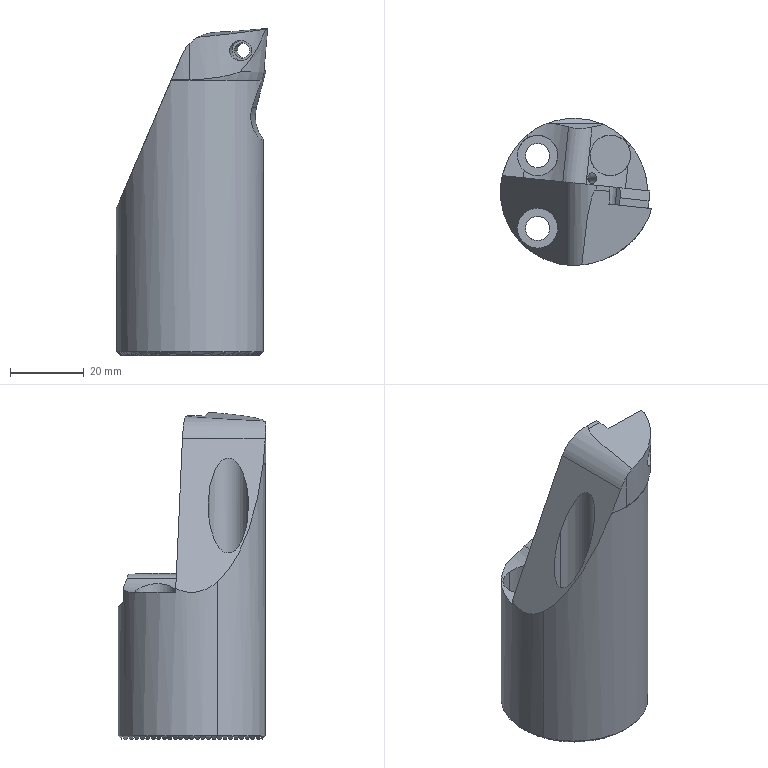NC program | Mastercam | posted with a generic post
Whole program:
%
:0001()
(MATERIAL - ALUMINUM MM - 2024)
(T10|50 FM/CTM |H10)
(T2|12 FEMR |H2|D2|WEAR COMP|TOOL DIA. - 12.|XY STOCK TO LEAVE - .3|Z STOCK TO LEAVE - 0.)
(T3|10 CHM |H3)
(T4|11 DR |H4)
(T11|6.6 DR |H11)
(T7|6 CBCHM |H7|D7|WEAR COMP|TOOL DIA. - 6.)
(T5|8 FEMR |H5|D5|WEAR COMP|TOOL DIA. - 8.|XY STOCK TO LEAVE - .05|Z STOCK TO LEAVE - .05)
(T6|8 FEMF |H6|D6|WEAR COMP|TOOL DIA. - 8.|XY STOCK TO LEAVE - .01|Z STOCK TO LEAVE - 0.)
(T8|26 60DTH |H8|D8|WEAR COMP|TOOL DIA. - 26.|XY STOCK TO LEAVE - .1|Z STOCK TO LEAVE - 0.)
(T13|11 DR |H13)
(T12|10.8 FL |H12)
N100 G21
N102 G0 G17 G40 G80 G90 G94 G98
N104 G0 G28 G91 Z0.
N106 G0 G28 X0. Y0.
(50 FM/CTM |TOOL - 10|DIA. OFF. - 10|LEN. - 10|TOOL DIA. - 50.)
N108 T10 M6
N110 G0 G54 G90 X0. Y-55. C0. B0. S1600 M3
N112 G43 H10 Z53.5
N114 Z4.5
N116 G1 Z0. F600.
N118 Y-20.
N120 Y20.
N122 Y55.
N124 G0 Z53.5
N126 M5
N128 G0 G28 G91 Z0.
N130 G28
N132 M01
N134 G0 G17 G40 G80 G90 G94 G98
N136 G0 G28 G91 Z0.
(12 FEMR |TOOL - 2|DIA. OFF. - 2|LEN. - 2|TOOL DIA. - 12.)
N138 T2 M6
N140 G0 G54 G90 X-1. Y35.7 C0. B0. S3500 M3
N142 G43 H2 Z50.
N144 Z1.
N146 G1 Z-1.5 F2000.
N148 G41 D2 Y27.3 F400.
N150 G3 X0. Y26.3 I1.
N152 G2 X26.3 Y0. J-26.3
N154 X0. Y-26.3 I-26.3
N156 X-26.3 Y0. J26.3
N158 X0. Y26.3 I26.3
N160 X.5 Y26.295 J-26.3
N162 G1 X.519
N164 G3 X1.519 Y27.276 J1.
N166 G1 G40 X1.678 Y35.675
N168 G0 Z50.
N170 M5
N172 G0 G28 G91 Z0.
N174 G28
N176 M01
N178 G0 G17 G40 G80 G90 G94 G98
N180 G0 G28 G91 Z0.
(10 CHM |TOOL - 3|DIA. OFF. - 3|LEN. - 3|TOOL DIA. - 10.)
N182 T3 M6
N184 G0 G54 G90 X9.899 Y-9.899 C0. B0. S2000 M3
N186 G43 H3 Z50.
N188 G81 G98 Z-3.8 R1. F100.
N190 Y9.899
N192 X-9.899
N194 X0. Y0. Z-1.
N196 G80
N198 M5
N200 G0 G28 G91 Z0.
N202 G28
N204 M01
N206 G0 G17 G40 G80 G90 G94 G98
N208 G0 G28 G91 Z0.
(11 DR |TOOL - 4|DIA. OFF. - 4|LEN. - 4|TOOL DIA. - 11.)
N210 T4 M6
N212 G0 G54 G90 X0. Y0. C0. B0. S2000 M3
N214 G43 H4 Z50.
N216 G83 G98 Z-9.5 R1. Q4. F80.
N218 G80
N220 M5
N222 G0 G28 G91 Z0.
N224 G28
N226 M01
N228 G0 G17 G40 G80 G90 G94 G98
N230 G0 G28 G91 Z0.
(6.6 DR |TOOL - 11|DIA. OFF. - 11|LEN. - 11|TOOL DIA. - 6.6)
N232 T11 M6
N234 G0 G54 G90 X-9.899 Y9.899 C0. B0. S2300 M3
N236 G43 H11 Z50.
N238 G81 G98 Z-9. R2. F60.
N240 X9.899
N242 Y-9.899
N244 G80
N246 M5
N248 G0 G28 G91 Z0.
N250 G28
N252 M01
N254 G0 G17 G40 G80 G90 G94 G98
N256 G0 G28 G91 Z0.
(6 CBCHM |TOOL - 7|DIA. OFF. - 7|LEN. - 7|TOOL DIA. - 6.)
N258 T7 M6
N260 G0 G54 G90 X-25.192 Y-.806 C0. B0. S3500 M3
N262 G43 H7 Z50.
N264 Z1.
N266 G1 Z-1.2 F2000.
N268 G41 D7 X-20.992 Y-.755 F400.
N270 G3 X-20.498 Y-.255 I-.006 J.5
N272 G1 Y-.249
N274 G2 X-20.5 Y0. I20.498 J.249
N276 X0. Y20.5 I20.5
N278 X20.5 Y0. J-20.5
N280 X0. Y-20.5 I-20.5
N282 X-20.498 Y-.249 J20.5
N284 X-20.5 Y0. I20.498 J.249
N286 X-20.498 Y.251 I20.5
N288 G1 Y.257
N290 G3 X-20.992 Y.757 I-.5
N292 G1 G40 X-25.192 Y.809
N294 G0 Z50.
N296 X2.529 Y.324
N298 Z1.
N300 G1 Z-1.8 F2000.
N302 G41 D7 X4.424 Y.963 F400.
N304 G3 X4.764 Y1.437 I-.16 J.474
N306 X4.738 Y1.596 I-.5
N308 X0. Y5. I-4.738 J-1.596
N310 X-5. Y0. J-5.
N312 X0. Y-5. I5.
N314 X5. Y0. J5.
N316 X4.738 Y1.596 I-5.
N318 X4.555 Y2.062 I-4.738 J-1.596
N320 X4.1 Y2.355 I-.455 J-.207
N322 X3.894 Y2.311 J-.5
N324 G1 G40 X2.071 Y1.486
N326 G0 Z50.
N328 M5
N330 G0 G28 G91 Z0.
N332 G28
N334 M01
N336 G0 G17 G40 G80 G90 G94 G98
N338 G0 G28 G91 Z0.
(8 FEMR |TOOL - 5|DIA. OFF. - 5|LEN. - 5|TOOL DIA. - 8.)
N340 T5 M6
N342 G0 G54 G90 X0. Y0. C0. B0. S3500 M3
N344 G43 H5 Z50.
N346 Z2.
N348 G1 Z-3.95 F2000.
N350 G41 D5 X-1.363 F400.
N352 G3 X-1.407 Y-.248 I.682 J-.248
N354 X-1.363 Y-.496 I.726
N356 X0. Y-1.45 I1.363 J.496
N358 X1.45 Y0. J1.45
N360 X0. Y1.45 I-1.45
N362 X-1.45 Y0. J-1.45
N364 X-1.363 Y-.496 I1.45
N366 X-1.311 Y-.619 I1.363 J.496
N368 X-.959 Y-.968 I.655 J.31
N370 G1 G40 X0. Y0.
N372 G41 D5 X-1.597
N374 G3 X-1.648 Y-.291 I.798 J-.291
N376 X-1.597 Y-.581 I.849
N378 X0. Y-1.699 I1.597 J.581
N380 X1.699 Y0. J1.699
N382 X0. Y1.699 I-1.699
N384 X-1.699 Y0. J-1.699
N386 X-1.597 Y-.581 I1.699
N388 X-1.54 Y-.719 I1.597 J.581
N390 X-1.129 Y-1.13 I.77 J.359
N392 G1 G40 X0. Y0.
N394 G41 D5 X-1.832
N396 G3 X-1.891 Y-.333 I.916 J-.333
N398 X-1.832 Y-.667 I.975
N400 X0. Y-1.95 I1.832 J.667
N402 X1.95 Y0. J1.95
N404 X0. Y1.95 I-1.95
N406 X-1.95 Y0. J-1.95
N408 X-1.832 Y-.667 I1.95
N410 X-1.77 Y-.818 I1.832 J.667
N412 X-1.3 Y-1.292 I.885 J.409
N414 G1 G40 X0. Y0.
N416 G0 Z50.
N418 M5
N420 G0 G28 G91 Z0.
N422 G28
N424 M01
N426 G0 G17 G40 G80 G90 G94 G98
N428 G0 G28 G91 Z0.
(8 FEMF |TOOL - 6|DIA. OFF. - 6|LEN. - 6|TOOL DIA. - 8.)
N430 T6 M6
N432 G0 G54 G90 X0. Y0. C0. B0. S3500 M3
N434 G43 H6 Z50.
N436 Z2.
N438 G1 Z-4. F2000.
N440 G41 D6 X-1.87 F400.
N442 G3 X-1.93 Y-.34 I.935 J-.34
N444 X-1.87 Y-.681 I.995
N446 X0. Y-1.99 I1.87 J.681
N448 X1.99 Y0. J1.99
N450 X0. Y1.99 I-1.99
N452 X-1.99 Y0. J-1.99
N454 X-1.87 Y-.681 I1.99
N456 X-1.807 Y-.834 I1.87 J.681
N458 X-1.327 Y-1.317 I.904 J.417
N460 G1 G40 X0. Y0.
N462 G41 D6 X-1.87
N464 G3 X-1.93 Y-.34 I.935 J-.34
N466 X-1.87 Y-.681 I.995
N468 X0. Y-1.99 I1.87 J.681
N470 X1.99 Y0. J1.99
N472 X0. Y1.99 I-1.99
N474 X-1.99 Y0. J-1.99
N476 X-1.87 Y-.681 I1.99
N478 X-1.807 Y-.834 I1.87 J.681
N480 X-1.327 Y-1.317 I.904 J.417
N482 G1 G40 X0. Y0.
N484 G41 D6 X-1.87
N486 G3 X-1.93 Y-.34 I.935 J-.34
N488 X-1.87 Y-.681 I.995
N490 X0. Y-1.99 I1.87 J.681
N492 X1.99 Y0. J1.99
N494 X0. Y1.99 I-1.99
N496 X-1.99 Y0. J-1.99
N498 X-1.87 Y-.681 I1.99
N500 X-1.807 Y-.834 I1.87 J.681
N502 X-1.327 Y-1.317 I.904 J.417
N504 G1 G40 X0. Y0.
N506 G0 Z50.
N508 M5
N510 G0 G28 G91 Z0.
N512 G28
N514 M01
N516 G0 G17 G40 G80 G90 G94 G98
N518 G0 G28 G91 Z0.
(50 FM/CTM |TOOL - 10|DIA. OFF. - 10|LEN. - 10|TOOL DIA. - 50.)
N520 T10 M6
N522 G0 G54 G90 X0. Y-55. C0. B0. S1600 M3
N524 G43 H10 Z53.5
N526 Z4.5
N528 G1 Z0. F600.
N530 Y-20.
N532 Y20.
N534 Y55.
N536 G0 Z53.5
N538 M5
N540 G0 G28 G91 Z0.
N542 G28
N544 M01
N546 G0 G17 G40 G80 G90 G94 G98
N548 G0 G28 G91 Z0.
(12 FEMR |TOOL - 2|DIA. OFF. - 2|LEN. - 2|TOOL DIA. - 12.)
N550 T2 M6
N552 G0 G54 G90 X-.747 Y35.706 C0. B0. S3500 M3
N554 G43 H2 Z50.
N556 Z1.
N558 G1 Z-1.5 F2000.
N560 G41 D2 X-.806 Y27.306 F400.
N562 Y27.299
N564 G3 X.187 Y26.299 I1.
N566 G2 X26.3 Y0. I-.187 J-26.299
N568 X0. Y-26.3 I-26.3
N570 X-26.3 Y0. J26.3
N572 X0. Y26.3 I26.3
N574 X.187 Y26.299 J-26.3
N576 X.687 Y26.291 I-.187 J-26.299
N578 G1 X.713
N580 G3 X1.712 Y27.265 J1.
N582 G1 G40 X1.932 Y35.662
N584 G0 Z50.
N586 M5
N588 G0 G28 G91 Z0.
N590 G28
N592 M01
N594 G0 G17 G40 G80 G90 G94 G98
N596 G0 G28 G91 Z0.
(10 CHM |TOOL - 3|DIA. OFF. - 3|LEN. - 3|TOOL DIA. - 10.)
N598 T3 M6
N600 G0 G54 G90 X9.899 Y-9.899 C0. B0. S2000 M3
N602 G43 H3 Z50.
N604 G81 G98 Z-3.8 R1. F100.
N606 Y9.899
N608 X-9.899
N610 G80
N612 M5
N614 G0 G28 G91 Z0.
N616 G28
N618 M01
N620 G0 G17 G40 G80 G90 G94 G98
N622 G0 G28 G91 Z0.
(6.6 DR |TOOL - 11|DIA. OFF. - 11|LEN. - 11|TOOL DIA. - 6.6)
N624 T11 M6
N626 G0 G54 G90 X-9.899 Y9.899 C0. B0. S2300 M3
N628 G43 H11 Z50.
N630 G81 G98 Z-9. R2. F60.
N632 X9.899
N634 Y-9.899
N636 G80
N638 M5
N640 G0 G28 G91 Z0.
N642 G28
N644 M01
N646 G0 G17 G40 G80 G90 G94 G98
N648 G0 G28 G91 Z0.
(11 DR |TOOL - 4|DIA. OFF. - 4|LEN. - 4|TOOL DIA. - 11.)
N650 T4 M6
N652 G0 G54 G90 X0. Y0. C0. B0. S2000 M3
N654 G43 H4 Z50.
N656 G83 G98 Z-14.805 R1. Q4. F80.
N658 G80
N660 M5
N662 G0 G28 G91 Z0.
N664 G28
N666 M01
N668 G0 G17 G40 G80 G90 G94 G98
N670 G0 G28 G91 Z0.
(6 CBCHM |TOOL - 7|DIA. OFF. - 7|LEN. - 7|TOOL DIA. - 6.)
N672 T7 M6
N674 G0 G54 G90 X-.5 Y25.2 C0. B0. S3500 M3
N676 G43 H7 Z50.
N678 Z1.
N680 G1 Z-1.2 F2000.
N682 G41 D7 Y21. F400.
N684 G3 X0. Y20.5 I.5
N686 G2 X20.5 Y0. J-20.5
N688 X0. Y-20.5 I-20.5
N690 X-20.5 Y0. J20.5
N692 X0. Y20.5 I20.5
N694 X.5 Y20.494 J-20.5
N696 G1 X.512
N698 G3 X1.012 Y20.982 J.5
N700 G1 G40 X1.114 Y25.18
N702 G0 Z50.
N704 X2.529 Y.324
N706 Z1.
N708 G1 Z-1.8 F2000.
N710 G41 D7 X4.424 Y.963 F400.
N712 G3 X4.764 Y1.437 I-.16 J.474
N714 X4.738 Y1.596 I-.5
N716 X0. Y5. I-4.738 J-1.596
N718 X-5. Y0. J-5.
N720 X0. Y-5. I5.
N722 X5. Y0. J5.
N724 X4.738 Y1.596 I-5.
N726 X4.555 Y2.062 I-4.738 J-1.596
N728 X4.1 Y2.355 I-.455 J-.207
N730 X3.894 Y2.311 J-.5
N732 G1 G40 X2.071 Y1.486
N734 G0 Z50.
N736 M5
N738 G0 G28 G91 Z0.
N740 G28
N742 M01
N744 G0 G17 G40 G80 G90 G94 G98
N746 G0 G28 G91 Z0.
(8 FEMR |TOOL - 5|DIA. OFF. - 5|LEN. - 5|TOOL DIA. - 8.)
N748 T5 M6
N750 G0 G54 G90 X0. Y0. C0. B0. S3500 M3
N752 G43 H5 Z50.
N754 Z2.
N756 G1 Z-3.95 F2000.
N758 G41 D5 X-1.363 F400.
N760 G3 X-1.407 Y-.248 I.682 J-.248
N762 X-1.363 Y-.496 I.726
N764 X0. Y-1.45 I1.363 J.496
N766 X1.45 Y0. J1.45
N768 X0. Y1.45 I-1.45
N770 X-1.45 Y0. J-1.45
N772 X-1.363 Y-.496 I1.45
N774 X-1.311 Y-.619 I1.363 J.496
N776 X-.959 Y-.968 I.655 J.31
N778 G1 G40 X0. Y0.
N780 G41 D5 X-1.597
N782 G3 X-1.648 Y-.291 I.798 J-.291
N784 X-1.597 Y-.581 I.849
N786 X0. Y-1.699 I1.597 J.581
N788 X1.699 Y0. J1.699
N790 X0. Y1.699 I-1.699
N792 X-1.699 Y0. J-1.699
N794 X-1.597 Y-.581 I1.699
N796 X-1.54 Y-.719 I1.597 J.581
N798 X-1.129 Y-1.13 I.77 J.359
N800 G1 G40 X0. Y0.
N802 G41 D5 X-1.832
N804 G3 X-1.891 Y-.333 I.916 J-.333
N806 X-1.832 Y-.667 I.975
N808 X0. Y-1.95 I1.832 J.667
N810 X1.95 Y0. J1.95
N812 X0. Y1.95 I-1.95
N814 X-1.95 Y0. J-1.95
N816 X-1.832 Y-.667 I1.95
N818 X-1.77 Y-.818 I1.832 J.667
N820 X-1.3 Y-1.292 I.885 J.409
N822 G1 G40 X0. Y0.
N824 G0 Z50.
N826 M5
N828 G0 G28 G91 Z0.
N830 G28
N832 M01
N834 G0 G17 G40 G80 G90 G94 G98
N836 G0 G28 G91 Z0.
(8 FEMF |TOOL - 6|DIA. OFF. - 6|LEN. - 6|TOOL DIA. - 8.)
N838 T6 M6
N840 G0 G54 G90 X0. Y0. C0. B0. S3500 M3
N842 G43 H6 Z50.
N844 Z2.
N846 G1 Z-4. F2000.
N848 G41 D6 X-1.87 F400.
N850 G3 X-1.93 Y-.34 I.935 J-.34
N852 X-1.87 Y-.681 I.995
N854 X0. Y-1.99 I1.87 J.681
N856 X1.99 Y0. J1.99
N858 X0. Y1.99 I-1.99
N860 X-1.99 Y0. J-1.99
N862 X-1.87 Y-.681 I1.99
N864 X-1.807 Y-.834 I1.87 J.681
N866 X-1.327 Y-1.317 I.904 J.417
N868 G1 G40 X0. Y0.
N870 G41 D6 X-1.87
N872 G3 X-1.93 Y-.34 I.935 J-.34
N874 X-1.87 Y-.681 I.995
N876 X0. Y-1.99 I1.87 J.681
N878 X1.99 Y0. J1.99
N880 X0. Y1.99 I-1.99
N882 X-1.99 Y0. J-1.99
N884 X-1.87 Y-.681 I1.99
N886 X-1.807 Y-.834 I1.87 J.681
N888 X-1.327 Y-1.317 I.904 J.417
N890 G1 G40 X0. Y0.
N892 G41 D6 X-1.87
N894 G3 X-1.93 Y-.34 I.935 J-.34
N896 X-1.87 Y-.681 I.995
N898 X0. Y-1.99 I1.87 J.681
N900 X1.99 Y0. J1.99
N902 X0. Y1.99 I-1.99
N904 X-1.99 Y0. J-1.99
N906 X-1.87 Y-.681 I1.99
N908 X-1.807 Y-.834 I1.87 J.681
N910 X-1.327 Y-1.317 I.904 J.417
N912 G1 G40 X0. Y0.
N914 G0 Z50.
N916 M5
N918 G0 G28 G91 Z0.
N920 G28
N922 M01
N924 G0 G17 G40 G80 G90 G94 G98
N926 G0 G28 G91 Z0.
(26 60DTH |TOOL - 8|DIA. OFF. - 8|LEN. - 8|TOOL DIA. - 26.)
N928 T8 M6
N930 G0 G54 G90 X17.749 Y11.176 C0. B-90. S4000 M3
N932 G43 H8 Z68.75
N934 Z19.75
N936 G1 Z13.75 F2000.
N938 G41 D8 X12.82 F1000.
N940 G3 X12.3 Y10.656 J-.52
N942 G1 Y6.96
N944 Y-6.96
N946 Y-10.656
N948 G3 X12.82 Y-11.176 I.52
N950 G1 G40 X17.749
N952 G0 Z28.75
N954 Y14.338
N956 Z18.25
N958 G1 Z12.25 F2000.
N960 G41 D8 X12.82 F1000.
N962 G3 X12.3 Y13.818 J-.52
N964 G1 Y10.121
N966 Y-10.121
N968 Y-13.818
N970 G3 X12.82 Y-14.338 I.52
N972 G1 G40 X17.749
N974 G0 Z27.25
N976 Y16.543
N978 Z16.75
N980 G1 Z10.75 F2000.
N982 G41 D8 X12.82 F1000.
N984 G3 X12.3 Y16.023 J-.52
N986 G1 Y12.326
N988 Y-12.326
N990 Y-16.023
N992 G3 X12.82 Y-16.543 I.52
N994 G1 G40 X17.749
N996 G0 Z25.75
N998 Y18.25
N1000 Z15.25
N1002 G1 Z9.25 F2000.
N1004 G41 D8 X12.82 F1000.
N1006 G3 X12.3 Y17.73 J-.52
N1008 G1 Y14.033
N1010 Y-14.033
N1012 Y-17.73
N1014 G3 X12.82 Y-18.25 I.52
N1016 G1 G40 X17.749
N1018 G0 Z24.25
N1020 Y19.626
N1022 Z13.75
N1024 G1 Z7.75 F2000.
N1026 G41 D8 X12.82 F1000.
N1028 G3 X12.3 Y19.106 J-.52
N1030 G1 Y15.409
N1032 Y-15.409
N1034 Y-19.106
N1036 G3 X12.82 Y-19.626 I.52
N1038 G1 G40 X17.749
N1040 G0 Z22.75
N1042 Y20.753
N1044 Z12.25
N1046 G1 Z6.25 F2000.
N1048 G41 D8 X12.82 F1000.
N1050 G3 X12.3 Y20.233 J-.52
N1052 G1 Y16.536
N1054 Y-16.536
N1056 Y-20.233
N1058 G3 X12.82 Y-20.753 I.52
N1060 G1 G40 X17.749
N1062 G0 Z21.25
N1064 Y21.679
N1066 Z10.75
N1068 G1 Z4.75 F2000.
N1070 G41 D8 X12.82 F1000.
N1072 G3 X12.3 Y21.159 J-.52
N1074 G1 Y17.462
N1076 Y-17.462
N1078 Y-21.159
N1080 G3 X12.82 Y-21.679 I.52
N1082 G1 G40 X17.749
N1084 G0 Z19.75
N1086 Y22.436
N1088 Z9.25
N1090 G1 Z3.25 F2000.
N1092 G41 D8 X12.82 F1000.
N1094 G3 X12.3 Y21.916 J-.52
N1096 G1 Y18.219
N1098 Y-18.219
N1100 Y-21.916
N1102 G3 X12.82 Y-22.436 I.52
N1104 G1 G40 X17.749
N1106 G0 Z18.25
N1108 Y23.043
N1110 Z7.75
N1112 G1 Z1.75 F2000.
N1114 G41 D8 X12.82 F1000.
N1116 G3 X12.3 Y22.523 J-.52
N1118 G1 Y18.827
N1120 Y-18.827
N1122 Y-22.523
N1124 G3 X12.82 Y-23.043 I.52
N1126 G1 G40 X17.749
N1128 G0 Z16.75
N1130 Y23.515
N1132 Z6.25
N1134 G1 Z.25 F2000.
N1136 G41 D8 X12.82 F1000.
N1138 G3 X12.3 Y22.995 J-.52
N1140 G1 Y19.299
N1142 Y-19.299
N1144 Y-22.995
N1146 G3 X12.82 Y-23.515 I.52
N1148 G1 G40 X17.749
N1150 G0 Z15.25
N1152 Y23.862
N1154 Z4.75
N1156 G1 Z-1.25 F2000.
N1158 G41 D8 X12.82 F1000.
N1160 G3 X12.3 Y23.342 J-.52
N1162 G1 Y19.645
N1164 Y-19.645
N1166 Y-23.342
N1168 G3 X12.82 Y-23.862 I.52
N1170 G1 G40 X17.749
N1172 G0 Z13.75
N1174 Y24.09
N1176 Z3.25
N1178 G1 Z-2.75 F2000.
N1180 G41 D8 X12.82 F1000.
N1182 G3 X12.3 Y23.57 J-.52
N1184 G1 Y19.873
N1186 Y-19.873
N1188 Y-23.57
N1190 G3 X12.82 Y-24.09 I.52
N1192 G1 G40 X17.749
N1194 G0 Z12.25
N1196 Y24.203
N1198 Z1.75
N1200 G1 Z-4.25 F2000.
N1202 G41 D8 X12.82 F1000.
N1204 G3 X12.3 Y23.683 J-.52
N1206 G1 Y19.986
N1208 Y-19.986
N1210 Y-23.683
N1212 G3 X12.82 Y-24.203 I.52
N1214 G1 G40 X17.749
N1216 G0 Z10.75
N1218 Y24.203
N1220 Z.25
N1222 G1 Z-5.75 F2000.
N1224 G41 D8 X12.82 F1000.
N1226 G3 X12.3 Y23.683 J-.52
N1228 G1 Y19.986
N1230 Y-19.986
N1232 Y-23.683
N1234 G3 X12.82 Y-24.203 I.52
N1236 G1 G40 X17.749
N1238 G0 Z9.25
N1240 Y24.09
N1242 Z-1.25
N1244 G1 Z-7.25 F2000.
N1246 G41 D8 X12.82 F1000.
N1248 G3 X12.3 Y23.57 J-.52
N1250 G1 Y19.873
N1252 Y-19.873
N1254 Y-23.57
N1256 G3 X12.82 Y-24.09 I.52
N1258 G1 G40 X17.749
N1260 G0 Z7.75
N1262 Y23.862
N1264 Z-2.75
N1266 G1 Z-8.75 F2000.
N1268 G41 D8 X12.82 F1000.
N1270 G3 X12.3 Y23.342 J-.52
N1272 G1 Y19.645
N1274 Y-19.645
N1276 Y-23.342
N1278 G3 X12.82 Y-23.862 I.52
N1280 G1 G40 X17.749
N1282 G0 Z6.25
N1284 Y23.515
N1286 Z-4.25
N1288 G1 Z-10.25 F2000.
N1290 G41 D8 X12.82 F1000.
N1292 G3 X12.3 Y22.995 J-.52
N1294 G1 Y19.299
N1296 Y-19.299
N1298 Y-22.995
N1300 G3 X12.82 Y-23.515 I.52
N1302 G1 G40 X17.749
N1304 G0 Z4.75
N1306 Y23.043
N1308 Z-5.75
N1310 G1 Z-11.75 F2000.
N1312 G41 D8 X12.82 F1000.
N1314 G3 X12.3 Y22.523 J-.52
N1316 G1 Y18.827
N1318 Y-18.827
N1320 Y-22.523
N1322 G3 X12.82 Y-23.043 I.52
N1324 G1 G40 X17.749
N1326 G0 Z3.25
N1328 Y22.436
N1330 Z-7.25
N1332 G1 Z-13.25 F2000.
N1334 G41 D8 X12.82 F1000.
N1336 G3 X12.3 Y21.916 J-.52
N1338 G1 Y18.219
N1340 Y-18.219
N1342 Y-21.916
N1344 G3 X12.82 Y-22.436 I.52
N1346 G1 G40 X17.749
N1348 G0 Z1.75
N1350 Y21.679
N1352 Z-8.75
N1354 G1 Z-14.75 F2000.
N1356 G41 D8 X12.82 F1000.
N1358 G3 X12.3 Y21.159 J-.52
N1360 G1 Y17.462
N1362 Y-17.462
N1364 Y-21.159
N1366 G3 X12.82 Y-21.679 I.52
N1368 G1 G40 X17.749
N1370 G0 Z.25
N1372 Y20.753
N1374 Z-10.25
N1376 G1 Z-16.25 F2000.
N1378 G41 D8 X12.82 F1000.
N1380 G3 X12.3 Y20.233 J-.52
N1382 G1 Y16.536
N1384 Y-16.536
N1386 Y-20.233
N1388 G3 X12.82 Y-20.753 I.52
N1390 G1 G40 X17.749
N1392 G0 Z-1.25
N1394 Y19.626
N1396 Z-11.75
N1398 G1 Z-17.75 F2000.
N1400 G41 D8 X12.82 F1000.
N1402 G3 X12.3 Y19.106 J-.52
N1404 G1 Y15.409
N1406 Y-15.409
N1408 Y-19.106
N1410 G3 X12.82 Y-19.626 I.52
N1412 G1 G40 X17.749
N1414 G0 Z-2.75
N1416 Y18.25
N1418 Z-13.25
N1420 G1 Z-19.25 F2000.
N1422 G41 D8 X12.82 F1000.
N1424 G3 X12.3 Y17.73 J-.52
N1426 G1 Y14.033
N1428 Y-14.033
N1430 Y-17.73
N1432 G3 X12.82 Y-18.25 I.52
N1434 G1 G40 X17.749
N1436 G0 Z-4.25
N1438 Y16.543
N1440 Z-14.75
N1442 G1 Z-20.75 F2000.
N1444 G41 D8 X12.82 F1000.
N1446 G3 X12.3 Y16.023 J-.52
N1448 G1 Y12.326
N1450 Y-12.326
N1452 Y-16.023
N1454 G3 X12.82 Y-16.543 I.52
N1456 G1 G40 X17.749
N1458 G0 Z-5.75
N1460 Y14.338
N1462 Z-16.25
N1464 G1 Z-22.25 F2000.
N1466 G41 D8 X12.82 F1000.
N1468 G3 X12.3 Y13.818 J-.52
N1470 G1 Y10.121
N1472 Y-10.121
N1474 Y-13.818
N1476 G3 X12.82 Y-14.338 I.52
N1478 G1 G40 X17.749
N1480 G0 Z-7.25
N1482 Y11.176
N1484 Z-17.75
N1486 G1 Z-23.75 F2000.
N1488 G41 D8 X12.82 F1000.
N1490 G3 X12.3 Y10.656 J-.52
N1492 G1 Y6.96
N1494 Y-6.96
N1496 Y-10.656
N1498 G3 X12.82 Y-11.176 I.52
N1500 G1 G40 X17.749
N1502 G0 Z31.25
N1504 M5
N1506 G0 G28 G91 Z0.
N1508 G28 B0.
N1510 M01
N1512 G0 G17 G40 G80 G90 G94 G98
N1514 G0 G28 G91 Z0.
(10 CHM |TOOL - 3|DIA. OFF. - 3|LEN. - 3|TOOL DIA. - 10.)
N1516 T3 M6
N1518 G0 G54 G90 X9.899 Y9.899 C0. B180. S2000 M3
N1520 G43 H3 Z79.5
N1522 G81 G98 Z29.5 R34.5 F100.
N1524 X-9.899
N1526 Y-9.899
N1528 G80
N1530 M5
N1532 G0 G28 G91 Z0.
N1534 G28 B0.
N1536 M01
N1538 G0 G17 G40 G80 G90 G94 G98
N1540 G0 G28 G91 Z0.
(11 DR |TOOL - 13|DIA. OFF. - 13|LEN. - 13|TOOL DIA. - 11.)
N1542 T13 M6
N1544 G0 G54 G90 X9.899 Y9.899 C0. B180. S2000 M3
N1546 G43 H13 Z70.
N1548 G83 G98 Z3. R35.5 Q2.1 F60.
N1550 X-9.899
N1552 Y-9.899
N1554 G80
N1556 M5
N1558 G0 G28 G91 Z0.
N1560 G28 B0.
N1562 M01
N1564 G0 G17 G40 G80 G90 G94 G98
N1566 G0 G28 G91 Z0.
(10.8 FL |TOOL - 12|DIA. OFF. - 12|LEN. - 12|TOOL DIA. - 11.)
N1568 T12 M6
N1570 G0 G54 G90 X9.899 Y9.899 C0. B180. S800 M3
N1572 G43 H12 Z70.
N1574 G82 G98 Z4.5 R10.5 P1. F60.
N1576 X-9.899 P1.
N1578 Y-9.899 P1.
N1580 G80
N1582 M5
N1584 G0 G28 G91 Z0.
N1586 G0 G28 X0. Y0.
N1588 G28 B0.
N1590 M30
%